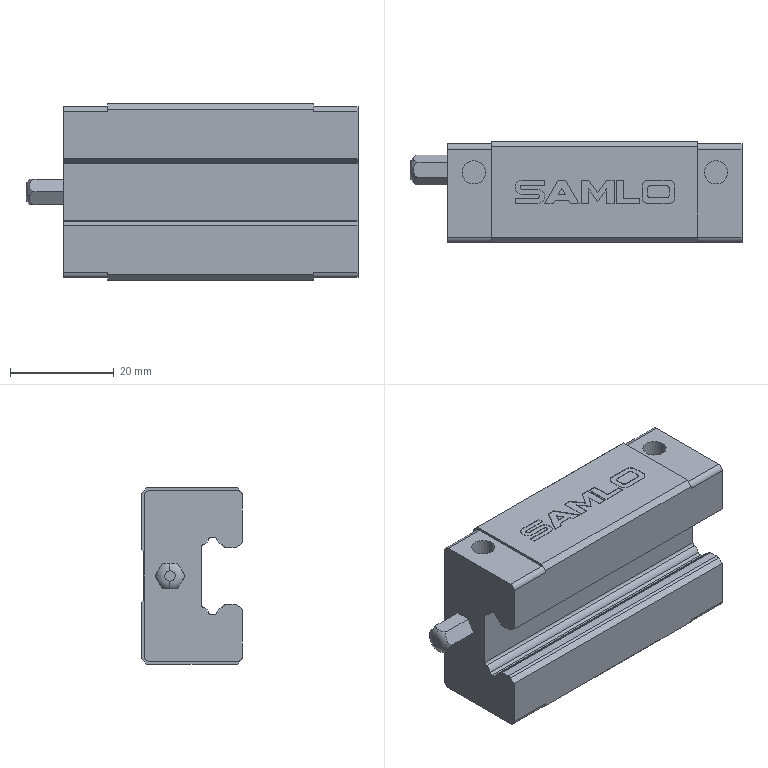Part | SolidWorks | features BaseBody 1 | 1 solid | 165 faces | box 64.1 x 19.5 x 34 mm | volume 30819 mm3 | plane 101 | cylinder 54 | cone 8 | torus 2 | commonest cylinder face diameters 1 x10 2 x10 3.242 x8 4.5 x8 1.045 x4 2.215 x4